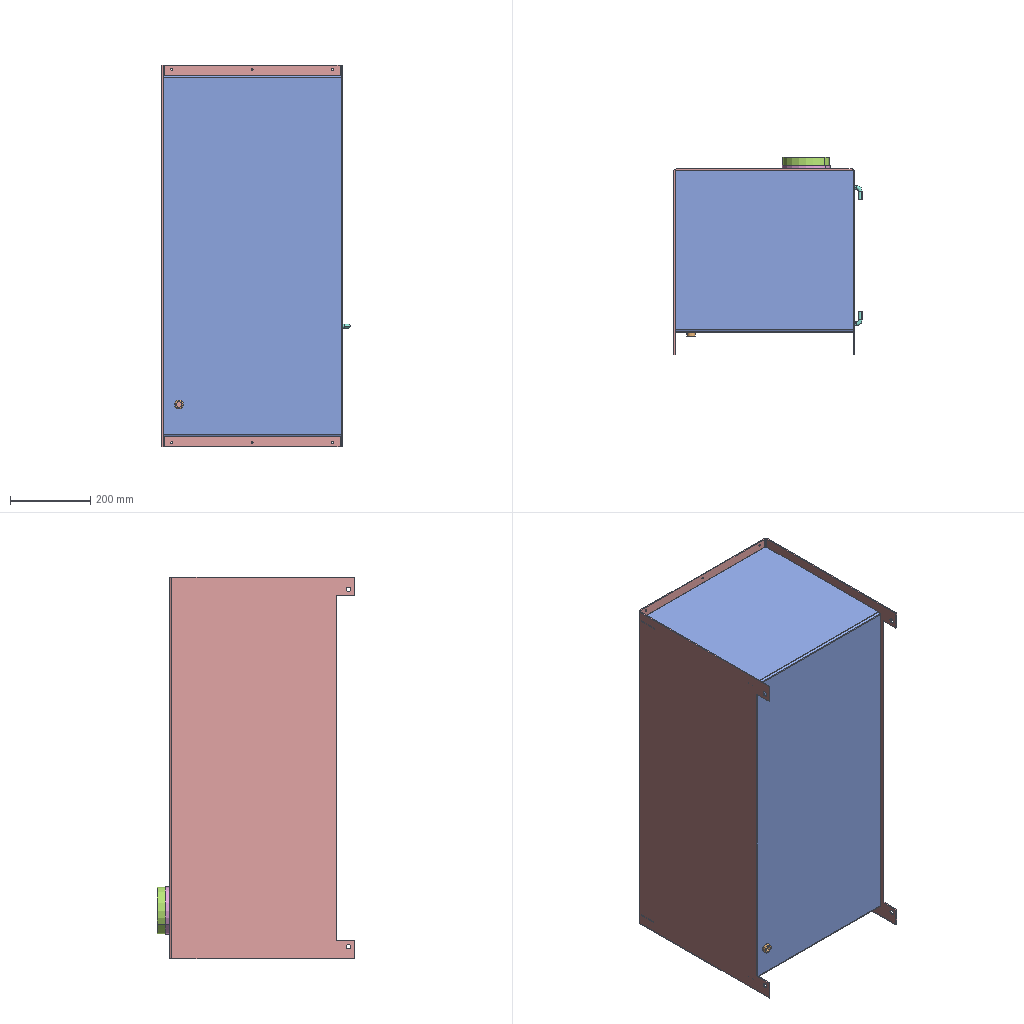Assembly | SolidWorks | 5 different items | 6 placed | box 469 x 491 x 950 mm
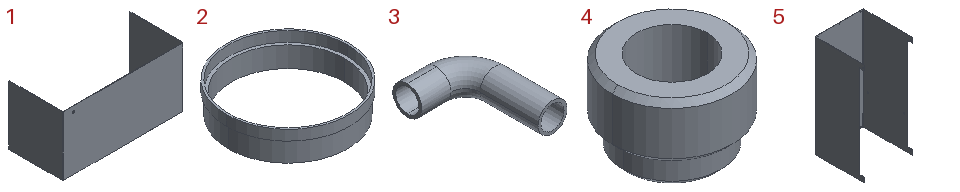Parts list (item | quantity | size | volume | features):
1 | x1 | 900 x 403 x 444 mm | 2258443 mm3 | features ICE 2, FlatPattern 1, SMBaseFlange 1, SheetMetal 1
2 | x1 | 120 x 120 x 30 mm | 28714 mm3 | features Extrusion 1, ICE 1
3 | x2 | 25 x 35 x 10 mm | 1292 mm3 | features Sweep 1
4 | x1 | 22 x 22 x 15 mm | 2988 mm3 | features ICE 2, Chamfer 1, Extrusion 1
5 | x1 | 450 x 461 x 950 mm | 3624099 mm3 | features ICE 3, FlatPattern 1, SMBaseFlange 1, SheetMetal 1
Mates (type | each side: item.copy, entity, surface, feature):
Coincident | 5.1 face plane Base-Flange1 | 1.1 face plane Base-Flange1 | 2 times
DistanceDim | 1.1 face plane Base-Flange1 | 5.1 face plane Base-Flange1
Concentric | 5.1 edge | 2.1 edge
Coincident | 5.1 face plane Base-Flange1 | 2.1 face plane Boss-Extrude2
Concentric | 5.1 edge | 3.1 edge
Parallel | 5.1 face plane Base-Flange1 | 3.1 face plane Sweep1
Concentric | 5.1 edge | 3.2 edge
Parallel | 3.1 face plane Sweep1 | 3.2 face plane Sweep1
Concentric | 1.1 edge | 4.1 edge
Coincident | 1.1 face plane Base-Flange1 | 4.1 face plane Cut-Extrude1